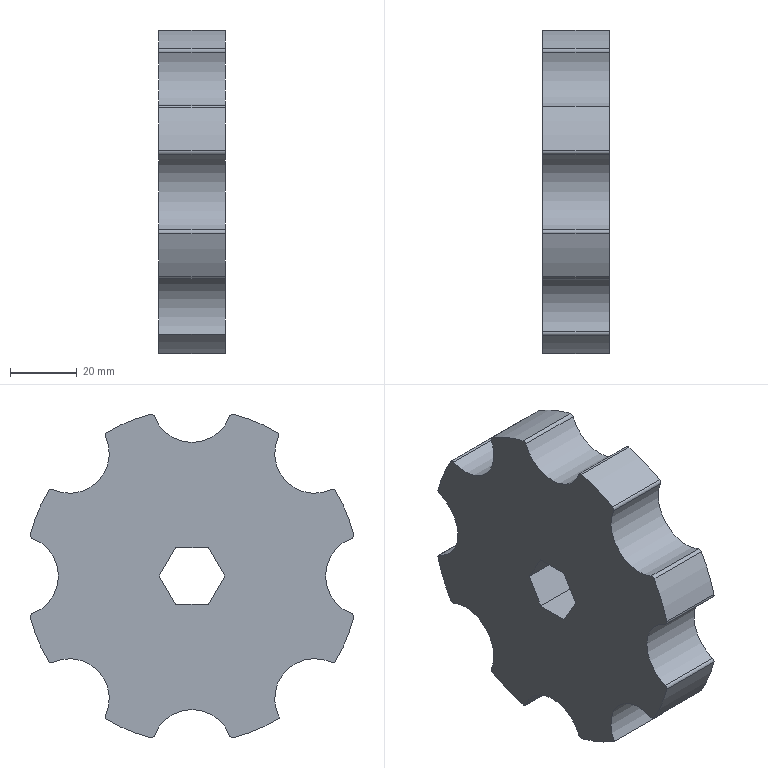Part | STEP file | Segmented slotted wheel | 1 solid | 39 faces | box 20 x 96.923 x 96.923 mm | volume 125193 mm3 | cylinder 31 | plane 8 | commonest cylinder face diameters 2 x15 24 x8 100 x8
STEP:
#1=CARTESIAN_POINT('',(20.,-48.43,-12.431));
#2=VERTEX_POINT('',#1);
#3=CARTESIAN_POINT('',(20.,-43.035,-25.455));
#4=VERTEX_POINT('',#3);
#5=CARTESIAN_POINT('',(20.,0.,0.));
#6=DIRECTION('',(1.,0.,0.));
#7=DIRECTION('',(0.,0.,-1.));
#8=AXIS2_PLACEMENT_3D('',#5,#6,#7);
#9=CIRCLE('',#8,50.);
#10=EDGE_CURVE('',#2,#4,#9,.T.);
#11=ORIENTED_EDGE('',*,*,#10,.T.);
#12=CARTESIAN_POINT('',(20.,-41.759,-25.856));
#13=VERTEX_POINT('',#12);
#14=CARTESIAN_POINT('',(20.,-42.174,-24.946));
#15=DIRECTION('',(1.,0.,0.));
#16=DIRECTION('',(0.,0.,-1.));
#17=AXIS2_PLACEMENT_3D('',#14,#15,#16);
#18=CIRCLE('',#17,1.);
#19=EDGE_CURVE('',#4,#13,#18,.T.);
#20=ORIENTED_EDGE('',*,*,#19,.T.);
#21=CARTESIAN_POINT('',(20.,-26.255,-42.552));
#22=VERTEX_POINT('',#21);
#23=CARTESIAN_POINT('',(20.,-36.77,-36.77));
#24=DIRECTION('',(-1.,0.,0.));
#25=DIRECTION('',(0.,0.,-1.));
#26=AXIS2_PLACEMENT_3D('',#23,#24,#25);
#27=CIRCLE('',#26,12.);
#28=EDGE_CURVE('',#13,#22,#27,.T.);
#29=ORIENTED_EDGE('',*,*,#28,.T.);
#30=CARTESIAN_POINT('',(20.,-12.431,-48.43));
#31=VERTEX_POINT('',#30);
#32=CARTESIAN_POINT('',(20.,0.,0.));
#33=DIRECTION('',(1.,0.,0.));
#34=DIRECTION('',(0.,0.,-1.));
#35=AXIS2_PLACEMENT_3D('',#32,#33,#34);
#36=CIRCLE('',#35,50.);
#37=EDGE_CURVE('',#22,#31,#36,.T.);
#38=ORIENTED_EDGE('',*,*,#37,.T.);
#39=CARTESIAN_POINT('',(20.,-11.245,-47.811));
#40=VERTEX_POINT('',#39);
#41=CARTESIAN_POINT('',(20.,-12.182,-47.462));
#42=DIRECTION('',(1.,0.,0.));
#43=DIRECTION('',(0.,0.,-1.));
#44=AXIS2_PLACEMENT_3D('',#41,#42,#43);
#45=CIRCLE('',#44,1.);
#46=EDGE_CURVE('',#31,#40,#45,.T.);
#47=ORIENTED_EDGE('',*,*,#46,.T.);
#48=CARTESIAN_POINT('',(20.,11.245,-47.811));
#49=VERTEX_POINT('',#48);
#50=CARTESIAN_POINT('',(20.,0.,-52.));
#51=DIRECTION('',(-1.,0.,0.));
#52=DIRECTION('',(0.,0.,-1.));
#53=AXIS2_PLACEMENT_3D('',#50,#51,#52);
#54=CIRCLE('',#53,12.);
#55=EDGE_CURVE('',#40,#49,#54,.T.);
#56=ORIENTED_EDGE('',*,*,#55,.T.);
#57=CARTESIAN_POINT('',(20.,12.431,-48.43));
#58=VERTEX_POINT('',#57);
#59=CARTESIAN_POINT('',(20.,12.182,-47.462));
#60=DIRECTION('',(1.,0.,0.));
#61=DIRECTION('',(0.,0.,-1.));
#62=AXIS2_PLACEMENT_3D('',#59,#60,#61);
#63=CIRCLE('',#62,1.);
#64=EDGE_CURVE('',#49,#58,#63,.T.);
#65=ORIENTED_EDGE('',*,*,#64,.T.);
#66=CARTESIAN_POINT('',(20.,25.455,-43.035));
#67=VERTEX_POINT('',#66);
#68=CARTESIAN_POINT('',(20.,0.,0.));
#69=DIRECTION('',(1.,0.,0.));
#70=DIRECTION('',(0.,0.,-1.));
#71=AXIS2_PLACEMENT_3D('',#68,#69,#70);
#72=CIRCLE('',#71,50.);
#73=EDGE_CURVE('',#58,#67,#72,.T.);
#74=ORIENTED_EDGE('',*,*,#73,.T.);
#75=CARTESIAN_POINT('',(20.,25.856,-41.759));
#76=VERTEX_POINT('',#75);
#77=CARTESIAN_POINT('',(20.,24.946,-42.174));
#78=DIRECTION('',(1.,0.,0.));
#79=DIRECTION('',(0.,0.,-1.));
#80=AXIS2_PLACEMENT_3D('',#77,#78,#79);
#81=CIRCLE('',#80,1.);
#82=EDGE_CURVE('',#67,#76,#81,.T.);
#83=ORIENTED_EDGE('',*,*,#82,.T.);
#84=CARTESIAN_POINT('',(20.,41.759,-25.856));
#85=VERTEX_POINT('',#84);
#86=CARTESIAN_POINT('',(20.,36.77,-36.77));
#87=DIRECTION('',(-1.,0.,0.));
#88=DIRECTION('',(0.,0.,-1.));
#89=AXIS2_PLACEMENT_3D('',#86,#87,#88);
#90=CIRCLE('',#89,12.);
#91=EDGE_CURVE('',#76,#85,#90,.T.);
#92=ORIENTED_EDGE('',*,*,#91,.T.);
#93=CARTESIAN_POINT('',(20.,43.035,-25.455));
#94=VERTEX_POINT('',#93);
#95=CARTESIAN_POINT('',(20.,42.174,-24.946));
#96=DIRECTION('',(1.,0.,0.));
#97=DIRECTION('',(0.,0.,-1.));
#98=AXIS2_PLACEMENT_3D('',#95,#96,#97);
#99=CIRCLE('',#98,1.);
#100=EDGE_CURVE('',#85,#94,#99,.T.);
#101=ORIENTED_EDGE('',*,*,#100,.T.);
#102=CARTESIAN_POINT('',(20.,48.43,-12.431));
#103=VERTEX_POINT('',#102);
#104=CARTESIAN_POINT('',(20.,0.,0.));
#105=DIRECTION('',(1.,0.,0.));
#106=DIRECTION('',(0.,0.,-1.));
#107=AXIS2_PLACEMENT_3D('',#104,#105,#106);
#108=CIRCLE('',#107,50.);
#109=EDGE_CURVE('',#94,#103,#108,.T.);
#110=ORIENTED_EDGE('',*,*,#109,.T.);
#111=CARTESIAN_POINT('',(20.,47.811,-11.245));
#112=VERTEX_POINT('',#111);
#113=CARTESIAN_POINT('',(20.,47.462,-12.182));
#114=DIRECTION('',(1.,0.,0.));
#115=DIRECTION('',(0.,0.,-1.));
#116=AXIS2_PLACEMENT_3D('',#113,#114,#115);
#117=CIRCLE('',#116,1.);
#118=EDGE_CURVE('',#103,#112,#117,.T.);
#119=ORIENTED_EDGE('',*,*,#118,.T.);
#120=CARTESIAN_POINT('',(20.,47.811,11.245));
#121=VERTEX_POINT('',#120);
#122=CARTESIAN_POINT('',(20.,52.,0.));
#123=DIRECTION('',(-1.,0.,0.));
#124=DIRECTION('',(0.,0.,-1.));
#125=AXIS2_PLACEMENT_3D('',#122,#123,#124);
#126=CIRCLE('',#125,12.);
#127=EDGE_CURVE('',#112,#121,#126,.T.);
#128=ORIENTED_EDGE('',*,*,#127,.T.);
#129=CARTESIAN_POINT('',(20.,48.43,12.431));
#130=VERTEX_POINT('',#129);
#131=CARTESIAN_POINT('',(20.,47.462,12.182));
#132=DIRECTION('',(1.,0.,0.));
#133=DIRECTION('',(0.,0.,-1.));
#134=AXIS2_PLACEMENT_3D('',#131,#132,#133);
#135=CIRCLE('',#134,1.);
#136=EDGE_CURVE('',#121,#130,#135,.T.);
#137=ORIENTED_EDGE('',*,*,#136,.T.);
#138=CARTESIAN_POINT('',(20.,43.035,25.455));
#139=VERTEX_POINT('',#138);
#140=CARTESIAN_POINT('',(20.,0.,0.));
#141=DIRECTION('',(1.,0.,0.));
#142=DIRECTION('',(0.,0.,-1.));
#143=AXIS2_PLACEMENT_3D('',#140,#141,#142);
#144=CIRCLE('',#143,50.);
#145=EDGE_CURVE('',#130,#139,#144,.T.);
#146=ORIENTED_EDGE('',*,*,#145,.T.);
#147=CARTESIAN_POINT('',(20.,41.759,25.856));
#148=VERTEX_POINT('',#147);
#149=CARTESIAN_POINT('',(20.,42.174,24.946));
#150=DIRECTION('',(1.,0.,0.));
#151=DIRECTION('',(0.,0.,-1.));
#152=AXIS2_PLACEMENT_3D('',#149,#150,#151);
#153=CIRCLE('',#152,1.);
#154=EDGE_CURVE('',#139,#148,#153,.T.);
#155=ORIENTED_EDGE('',*,*,#154,.T.);
#156=CARTESIAN_POINT('',(20.,25.856,41.759));
#157=VERTEX_POINT('',#156);
#158=CARTESIAN_POINT('',(20.,36.77,36.77));
#159=DIRECTION('',(-1.,0.,0.));
#160=DIRECTION('',(0.,0.,-1.));
#161=AXIS2_PLACEMENT_3D('',#158,#159,#160);
#162=CIRCLE('',#161,12.);
#163=EDGE_CURVE('',#148,#157,#162,.T.);
#164=ORIENTED_EDGE('',*,*,#163,.T.);
#165=CARTESIAN_POINT('',(20.,25.455,43.035));
#166=VERTEX_POINT('',#165);
#167=CARTESIAN_POINT('',(20.,24.946,42.174));
#168=DIRECTION('',(1.,0.,0.));
#169=DIRECTION('',(0.,0.,-1.));
#170=AXIS2_PLACEMENT_3D('',#167,#168,#169);
#171=CIRCLE('',#170,1.);
#172=EDGE_CURVE('',#157,#166,#171,.T.);
#173=ORIENTED_EDGE('',*,*,#172,.T.);
#174=CARTESIAN_POINT('',(20.,12.431,48.43));
#175=VERTEX_POINT('',#174);
#176=CARTESIAN_POINT('',(20.,0.,0.));
#177=DIRECTION('',(1.,0.,0.));
#178=DIRECTION('',(0.,0.,-1.));
#179=AXIS2_PLACEMENT_3D('',#176,#177,#178);
#180=CIRCLE('',#179,50.);
#181=EDGE_CURVE('',#166,#175,#180,.T.);
#182=ORIENTED_EDGE('',*,*,#181,.T.);
#183=CARTESIAN_POINT('',(20.,11.245,47.811));
#184=VERTEX_POINT('',#183);
#185=CARTESIAN_POINT('',(20.,12.182,47.462));
#186=DIRECTION('',(1.,0.,0.));
#187=DIRECTION('',(0.,0.,-1.));
#188=AXIS2_PLACEMENT_3D('',#185,#186,#187);
#189=CIRCLE('',#188,1.);
#190=EDGE_CURVE('',#175,#184,#189,.T.);
#191=ORIENTED_EDGE('',*,*,#190,.T.);
#192=CARTESIAN_POINT('',(20.,-11.245,47.811));
#193=VERTEX_POINT('',#192);
#194=CARTESIAN_POINT('',(20.,0.,52.));
#195=DIRECTION('',(-1.,0.,0.));
#196=DIRECTION('',(0.,0.,-1.));
#197=AXIS2_PLACEMENT_3D('',#194,#195,#196);
#198=CIRCLE('',#197,12.);
#199=EDGE_CURVE('',#184,#193,#198,.T.);
#200=ORIENTED_EDGE('',*,*,#199,.T.);
#201=CARTESIAN_POINT('',(20.,-12.431,48.43));
#202=VERTEX_POINT('',#201);
#203=CARTESIAN_POINT('',(20.,-12.182,47.462));
#204=DIRECTION('',(1.,0.,0.));
#205=DIRECTION('',(0.,0.,-1.));
#206=AXIS2_PLACEMENT_3D('',#203,#204,#205);
#207=CIRCLE('',#206,1.);
#208=EDGE_CURVE('',#193,#202,#207,.T.);
#209=ORIENTED_EDGE('',*,*,#208,.T.);
#210=CARTESIAN_POINT('',(20.,-25.455,43.035));
#211=VERTEX_POINT('',#210);
#212=CARTESIAN_POINT('',(20.,0.,0.));
#213=DIRECTION('',(1.,0.,0.));
#214=DIRECTION('',(0.,0.,-1.));
#215=AXIS2_PLACEMENT_3D('',#212,#213,#214);
#216=CIRCLE('',#215,50.);
#217=EDGE_CURVE('',#202,#211,#216,.T.);
#218=ORIENTED_EDGE('',*,*,#217,.T.);
#219=CARTESIAN_POINT('',(20.,-25.856,41.759));
#220=VERTEX_POINT('',#219);
#221=CARTESIAN_POINT('',(20.,-24.946,42.174));
#222=DIRECTION('',(1.,0.,0.));
#223=DIRECTION('',(0.,0.,-1.));
#224=AXIS2_PLACEMENT_3D('',#221,#222,#223);
#225=CIRCLE('',#224,1.);
#226=EDGE_CURVE('',#211,#220,#225,.T.);
#227=ORIENTED_EDGE('',*,*,#226,.T.);
#228=CARTESIAN_POINT('',(20.,-41.759,25.856));
#229=VERTEX_POINT('',#228);
#230=CARTESIAN_POINT('',(20.,-36.77,36.77));
#231=DIRECTION('',(-1.,0.,0.));
#232=DIRECTION('',(0.,0.,-1.));
#233=AXIS2_PLACEMENT_3D('',#230,#231,#232);
#234=CIRCLE('',#233,12.);
#235=EDGE_CURVE('',#220,#229,#234,.T.);
#236=ORIENTED_EDGE('',*,*,#235,.T.);
#237=CARTESIAN_POINT('',(20.,-43.035,25.455));
#238=VERTEX_POINT('',#237);
#239=CARTESIAN_POINT('',(20.,-42.174,24.946));
#240=DIRECTION('',(1.,0.,0.));
#241=DIRECTION('',(0.,0.,-1.));
#242=AXIS2_PLACEMENT_3D('',#239,#240,#241);
#243=CIRCLE('',#242,1.);
#244=EDGE_CURVE('',#229,#238,#243,.T.);
#245=ORIENTED_EDGE('',*,*,#244,.T.);
#246=CARTESIAN_POINT('',(20.,-48.43,12.431));
#247=VERTEX_POINT('',#246);
#248=CARTESIAN_POINT('',(20.,0.,0.));
#249=DIRECTION('',(1.,0.,0.));
#250=DIRECTION('',(0.,0.,-1.));
#251=AXIS2_PLACEMENT_3D('',#248,#249,#250);
#252=CIRCLE('',#251,50.);
#253=EDGE_CURVE('',#238,#247,#252,.T.);
#254=ORIENTED_EDGE('',*,*,#253,.T.);
#255=CARTESIAN_POINT('',(20.,-47.811,11.245));
#256=VERTEX_POINT('',#255);
#257=CARTESIAN_POINT('',(20.,-47.462,12.182));
#258=DIRECTION('',(1.,0.,0.));
#259=DIRECTION('',(0.,0.,-1.));
#260=AXIS2_PLACEMENT_3D('',#257,#258,#259);
#261=CIRCLE('',#260,1.);
#262=EDGE_CURVE('',#247,#256,#261,.T.);
#263=ORIENTED_EDGE('',*,*,#262,.T.);
#264=CARTESIAN_POINT('',(20.,-47.811,-11.245));
#265=VERTEX_POINT('',#264);
#266=CARTESIAN_POINT('',(20.,-52.,0.));
#267=DIRECTION('',(-1.,0.,0.));
#268=DIRECTION('',(0.,0.,-1.));
#269=AXIS2_PLACEMENT_3D('',#266,#267,#268);
#270=CIRCLE('',#269,12.);
#271=EDGE_CURVE('',#256,#265,#270,.T.);
#272=ORIENTED_EDGE('',*,*,#271,.T.);
#273=CARTESIAN_POINT('',(20.,-47.462,-12.182));
#274=DIRECTION('',(1.,0.,0.));
#275=DIRECTION('',(0.,0.,-1.));
#276=AXIS2_PLACEMENT_3D('',#273,#274,#275);
#277=CIRCLE('',#276,1.);
#278=EDGE_CURVE('',#265,#2,#277,.T.);
#279=ORIENTED_EDGE('',*,*,#278,.T.);
#280=EDGE_LOOP('',(#11,#20,#29,#38,#47,#56,#65,#74,#83,#92,#101,#110,#119,#128,#137,#146,#155,#164,#173,#182,#191,#200,#209,#218,#227,#236,#245,#254,#263,#272,#279));
#281=FACE_OUTER_BOUND('',#280,.T.);
#282=CARTESIAN_POINT('',(20.,9.815,0.));
#283=VERTEX_POINT('',#282);
#284=CARTESIAN_POINT('',(20.,4.907,8.5));
#285=VERTEX_POINT('',#284);
#286=CARTESIAN_POINT('',(20.,9.815,0.));
#287=DIRECTION('',(0.,-0.5,0.866));
#288=VECTOR('',#287,1000.);
#289=LINE('',#286,#288);
#290=EDGE_CURVE('',#283,#285,#289,.T.);
#291=ORIENTED_EDGE('',*,*,#290,.F.);
#292=CARTESIAN_POINT('',(20.,4.907,-8.5));
#293=VERTEX_POINT('',#292);
#294=CARTESIAN_POINT('',(20.,4.907,-8.5));
#295=DIRECTION('',(0.,0.5,0.866));
#296=VECTOR('',#295,1000.);
#297=LINE('',#294,#296);
#298=EDGE_CURVE('',#293,#283,#297,.T.);
#299=ORIENTED_EDGE('',*,*,#298,.F.);
#300=CARTESIAN_POINT('',(20.,-4.907,-8.5));
#301=VERTEX_POINT('',#300);
#302=CARTESIAN_POINT('',(20.,-4.907,-8.5));
#303=DIRECTION('',(0.,1.,0.));
#304=VECTOR('',#303,1000.);
#305=LINE('',#302,#304);
#306=EDGE_CURVE('',#301,#293,#305,.T.);
#307=ORIENTED_EDGE('',*,*,#306,.F.);
#308=CARTESIAN_POINT('',(20.,-9.815,0.));
#309=VERTEX_POINT('',#308);
#310=CARTESIAN_POINT('',(20.,-9.815,0.));
#311=DIRECTION('',(0.,0.5,-0.866));
#312=VECTOR('',#311,1000.);
#313=LINE('',#310,#312);
#314=EDGE_CURVE('',#309,#301,#313,.T.);
#315=ORIENTED_EDGE('',*,*,#314,.F.);
#316=CARTESIAN_POINT('',(20.,-4.907,8.5));
#317=VERTEX_POINT('',#316);
#318=CARTESIAN_POINT('',(20.,-4.907,8.5));
#319=DIRECTION('',(0.,-0.5,-0.866));
#320=VECTOR('',#319,1000.);
#321=LINE('',#318,#320);
#322=EDGE_CURVE('',#317,#309,#321,.T.);
#323=ORIENTED_EDGE('',*,*,#322,.F.);
#324=CARTESIAN_POINT('',(20.,4.907,8.5));
#325=DIRECTION('',(0.,-1.,0.));
#326=VECTOR('',#325,1000.);
#327=LINE('',#324,#326);
#328=EDGE_CURVE('',#285,#317,#327,.T.);
#329=ORIENTED_EDGE('',*,*,#328,.F.);
#330=EDGE_LOOP('',(#291,#299,#307,#315,#323,#329));
#331=FACE_BOUND('',#330,.T.);
#332=CARTESIAN_POINT('',(20.,26.,0.));
#333=DIRECTION('',(1.,0.,0.));
#334=DIRECTION('',(0.,0.,-1.));
#335=AXIS2_PLACEMENT_3D('',#332,#333,#334);
#336=PLANE('',#335);
#337=ADVANCED_FACE('',(#281,#331),#336,.T.);
#338=CARTESIAN_POINT('',(0.,-41.759,-25.856));
#339=VERTEX_POINT('',#338);
#340=CARTESIAN_POINT('',(0.,-26.255,-42.552));
#341=VERTEX_POINT('',#340);
#342=CARTESIAN_POINT('',(0.,-36.77,-36.77));
#343=DIRECTION('',(-1.,0.,0.));
#344=DIRECTION('',(0.,0.,-1.));
#345=AXIS2_PLACEMENT_3D('',#342,#343,#344);
#346=CIRCLE('',#345,12.);
#347=EDGE_CURVE('',#339,#341,#346,.T.);
#348=ORIENTED_EDGE('',*,*,#347,.F.);
#349=CARTESIAN_POINT('',(0.,-43.035,-25.455));
#350=VERTEX_POINT('',#349);
#351=CARTESIAN_POINT('',(0.,-42.174,-24.946));
#352=DIRECTION('',(-1.,0.,0.));
#353=DIRECTION('',(0.,0.,-1.));
#354=AXIS2_PLACEMENT_3D('',#351,#352,#353);
#355=CIRCLE('',#354,1.);
#356=EDGE_CURVE('',#339,#350,#355,.T.);
#357=ORIENTED_EDGE('',*,*,#356,.T.);
#358=CARTESIAN_POINT('',(0.,-48.43,-12.431));
#359=VERTEX_POINT('',#358);
#360=CARTESIAN_POINT('',(0.,0.,0.));
#361=DIRECTION('',(1.,0.,0.));
#362=DIRECTION('',(0.,0.,-1.));
#363=AXIS2_PLACEMENT_3D('',#360,#361,#362);
#364=CIRCLE('',#363,50.);
#365=EDGE_CURVE('',#359,#350,#364,.T.);
#366=ORIENTED_EDGE('',*,*,#365,.F.);
#367=CARTESIAN_POINT('',(0.,-47.811,-11.245));
#368=VERTEX_POINT('',#367);
#369=CARTESIAN_POINT('',(0.,-47.462,-12.182));
#370=DIRECTION('',(-1.,0.,0.));
#371=DIRECTION('',(0.,0.,-1.));
#372=AXIS2_PLACEMENT_3D('',#369,#370,#371);
#373=CIRCLE('',#372,1.);
#374=EDGE_CURVE('',#359,#368,#373,.T.);
#375=ORIENTED_EDGE('',*,*,#374,.T.);
#376=CARTESIAN_POINT('',(0.,-47.811,11.245));
#377=VERTEX_POINT('',#376);
#378=CARTESIAN_POINT('',(0.,-52.,0.));
#379=DIRECTION('',(-1.,0.,0.));
#380=DIRECTION('',(0.,0.,-1.));
#381=AXIS2_PLACEMENT_3D('',#378,#379,#380);
#382=CIRCLE('',#381,12.);
#383=EDGE_CURVE('',#377,#368,#382,.T.);
#384=ORIENTED_EDGE('',*,*,#383,.F.);
#385=CARTESIAN_POINT('',(0.,-48.43,12.431));
#386=VERTEX_POINT('',#385);
#387=CARTESIAN_POINT('',(0.,-47.462,12.182));
#388=DIRECTION('',(-1.,0.,0.));
#389=DIRECTION('',(0.,0.,-1.));
#390=AXIS2_PLACEMENT_3D('',#387,#388,#389);
#391=CIRCLE('',#390,1.);
#392=EDGE_CURVE('',#377,#386,#391,.T.);
#393=ORIENTED_EDGE('',*,*,#392,.T.);
#394=CARTESIAN_POINT('',(0.,-43.035,25.455));
#395=VERTEX_POINT('',#394);
#396=CARTESIAN_POINT('',(0.,0.,0.));
#397=DIRECTION('',(1.,0.,0.));
#398=DIRECTION('',(0.,0.,-1.));
#399=AXIS2_PLACEMENT_3D('',#396,#397,#398);
#400=CIRCLE('',#399,50.);
#401=EDGE_CURVE('',#395,#386,#400,.T.);
#402=ORIENTED_EDGE('',*,*,#401,.F.);
#403=CARTESIAN_POINT('',(0.,-41.759,25.856));
#404=VERTEX_POINT('',#403);
#405=CARTESIAN_POINT('',(0.,-42.174,24.946));
#406=DIRECTION('',(-1.,0.,0.));
#407=DIRECTION('',(0.,0.,-1.));
#408=AXIS2_PLACEMENT_3D('',#405,#406,#407);
#409=CIRCLE('',#408,1.);
#410=EDGE_CURVE('',#395,#404,#409,.T.);
#411=ORIENTED_EDGE('',*,*,#410,.T.);
#412=CARTESIAN_POINT('',(0.,-25.856,41.759));
#413=VERTEX_POINT('',#412);
#414=CARTESIAN_POINT('',(0.,-36.77,36.77));
#415=DIRECTION('',(-1.,0.,0.));
#416=DIRECTION('',(0.,0.,-1.));
#417=AXIS2_PLACEMENT_3D('',#414,#415,#416);
#418=CIRCLE('',#417,12.);
#419=EDGE_CURVE('',#413,#404,#418,.T.);
#420=ORIENTED_EDGE('',*,*,#419,.F.);
#421=CARTESIAN_POINT('',(0.,-25.455,43.035));
#422=VERTEX_POINT('',#421);
#423=CARTESIAN_POINT('',(0.,-24.946,42.174));
#424=DIRECTION('',(-1.,0.,0.));
#425=DIRECTION('',(0.,0.,-1.));
#426=AXIS2_PLACEMENT_3D('',#423,#424,#425);
#427=CIRCLE('',#426,1.);
#428=EDGE_CURVE('',#413,#422,#427,.T.);
#429=ORIENTED_EDGE('',*,*,#428,.T.);
#430=CARTESIAN_POINT('',(0.,-12.431,48.43));
#431=VERTEX_POINT('',#430);
#432=CARTESIAN_POINT('',(0.,0.,0.));
#433=DIRECTION('',(1.,0.,0.));
#434=DIRECTION('',(0.,0.,-1.));
#435=AXIS2_PLACEMENT_3D('',#432,#433,#434);
#436=CIRCLE('',#435,50.);
#437=EDGE_CURVE('',#431,#422,#436,.T.);
#438=ORIENTED_EDGE('',*,*,#437,.F.);
#439=CARTESIAN_POINT('',(0.,-11.245,47.811));
#440=VERTEX_POINT('',#439);
#441=CARTESIAN_POINT('',(0.,-12.182,47.462));
#442=DIRECTION('',(-1.,0.,0.));
#443=DIRECTION('',(0.,0.,-1.));
#444=AXIS2_PLACEMENT_3D('',#441,#442,#443);
#445=CIRCLE('',#444,1.);
#446=EDGE_CURVE('',#431,#440,#445,.T.);
#447=ORIENTED_EDGE('',*,*,#446,.T.);
#448=CARTESIAN_POINT('',(0.,11.245,47.811));
#449=VERTEX_POINT('',#448);
#450=CARTESIAN_POINT('',(0.,0.,52.));
#451=DIRECTION('',(-1.,0.,0.));
#452=DIRECTION('',(0.,0.,-1.));
#453=AXIS2_PLACEMENT_3D('',#450,#451,#452);
#454=CIRCLE('',#453,12.);
#455=EDGE_CURVE('',#449,#440,#454,.T.);
#456=ORIENTED_EDGE('',*,*,#455,.F.);
#457=CARTESIAN_POINT('',(0.,12.431,48.43));
#458=VERTEX_POINT('',#457);
#459=CARTESIAN_POINT('',(0.,12.182,47.462));
#460=DIRECTION('',(-1.,0.,0.));
#461=DIRECTION('',(0.,0.,-1.));
#462=AXIS2_PLACEMENT_3D('',#459,#460,#461);
#463=CIRCLE('',#462,1.);
#464=EDGE_CURVE('',#449,#458,#463,.T.);
#465=ORIENTED_EDGE('',*,*,#464,.T.);
#466=CARTESIAN_POINT('',(0.,25.455,43.035));
#467=VERTEX_POINT('',#466);
#468=CARTESIAN_POINT('',(0.,0.,0.));
#469=DIRECTION('',(1.,0.,0.));
#470=DIRECTION('',(0.,0.,-1.));
#471=AXIS2_PLACEMENT_3D('',#468,#469,#470);
#472=CIRCLE('',#471,50.);
#473=EDGE_CURVE('',#467,#458,#472,.T.);
#474=ORIENTED_EDGE('',*,*,#473,.F.);
#475=CARTESIAN_POINT('',(0.,25.856,41.759));
#476=VERTEX_POINT('',#475);
#477=CARTESIAN_POINT('',(0.,24.946,42.174));
#478=DIRECTION('',(-1.,0.,0.));
#479=DIRECTION('',(0.,0.,-1.));
#480=AXIS2_PLACEMENT_3D('',#477,#478,#479);
#481=CIRCLE('',#480,1.);
#482=EDGE_CURVE('',#467,#476,#481,.T.);
#483=ORIENTED_EDGE('',*,*,#482,.T.);
#484=CARTESIAN_POINT('',(0.,41.759,25.856));
#485=VERTEX_POINT('',#484);
#486=CARTESIAN_POINT('',(0.,36.77,36.77));
#487=DIRECTION('',(-1.,0.,0.));
#488=DIRECTION('',(0.,0.,-1.));
#489=AXIS2_PLACEMENT_3D('',#486,#487,#488);
#490=CIRCLE('',#489,12.);
#491=EDGE_CURVE('',#485,#476,#490,.T.);
#492=ORIENTED_EDGE('',*,*,#491,.F.);
#493=CARTESIAN_POINT('',(0.,43.035,25.455));
#494=VERTEX_POINT('',#493);
#495=CARTESIAN_POINT('',(0.,42.174,24.946));
#496=DIRECTION('',(-1.,0.,0.));
#497=DIRECTION('',(0.,0.,-1.));
#498=AXIS2_PLACEMENT_3D('',#495,#496,#497);
#499=CIRCLE('',#498,1.);
#500=EDGE_CURVE('',#485,#494,#499,.T.);
#501=ORIENTED_EDGE('',*,*,#500,.T.);
#502=CARTESIAN_POINT('',(0.,48.43,12.431));
#503=VERTEX_POINT('',#502);
#504=CARTESIAN_POINT('',(0.,0.,0.));
#505=DIRECTION('',(1.,0.,0.));
#506=DIRECTION('',(0.,0.,-1.));
#507=AXIS2_PLACEMENT_3D('',#504,#505,#506);
#508=CIRCLE('',#507,50.);
#509=EDGE_CURVE('',#503,#494,#508,.T.);
#510=ORIENTED_EDGE('',*,*,#509,.F.);
#511=CARTESIAN_POINT('',(0.,47.811,11.245));
#512=VERTEX_POINT('',#511);
#513=CARTESIAN_POINT('',(0.,47.462,12.182));
#514=DIRECTION('',(-1.,0.,0.));
#515=DIRECTION('',(0.,0.,-1.));
#516=AXIS2_PLACEMENT_3D('',#513,#514,#515);
#517=CIRCLE('',#516,1.);
#518=EDGE_CURVE('',#503,#512,#517,.T.);
#519=ORIENTED_EDGE('',*,*,#518,.T.);
#520=CARTESIAN_POINT('',(0.,47.811,-11.245));
#521=VERTEX_POINT('',#520);
#522=CARTESIAN_POINT('',(0.,52.,0.));
#523=DIRECTION('',(-1.,0.,0.));
#524=DIRECTION('',(0.,0.,-1.));
#525=AXIS2_PLACEMENT_3D('',#522,#523,#524);
#526=CIRCLE('',#525,12.);
#527=EDGE_CURVE('',#521,#512,#526,.T.);
#528=ORIENTED_EDGE('',*,*,#527,.F.);
#529=CARTESIAN_POINT('',(0.,48.43,-12.431));
#530=VERTEX_POINT('',#529);
#531=CARTESIAN_POINT('',(0.,47.462,-12.182));
#532=DIRECTION('',(-1.,0.,0.));
#533=DIRECTION('',(0.,0.,-1.));
#534=AXIS2_PLACEMENT_3D('',#531,#532,#533);
#535=CIRCLE('',#534,1.);
#536=EDGE_CURVE('',#521,#530,#535,.T.);
#537=ORIENTED_EDGE('',*,*,#536,.T.);
#538=CARTESIAN_POINT('',(0.,43.035,-25.455));
#539=VERTEX_POINT('',#538);
#540=CARTESIAN_POINT('',(0.,0.,0.));
#541=DIRECTION('',(1.,0.,0.));
#542=DIRECTION('',(0.,0.,-1.));
#543=AXIS2_PLACEMENT_3D('',#540,#541,#542);
#544=CIRCLE('',#543,50.);
#545=EDGE_CURVE('',#539,#530,#544,.T.);
#546=ORIENTED_EDGE('',*,*,#545,.F.);
#547=CARTESIAN_POINT('',(0.,41.759,-25.856));
#548=VERTEX_POINT('',#547);
#549=CARTESIAN_POINT('',(0.,42.174,-24.946));
#550=DIRECTION('',(-1.,0.,0.));
#551=DIRECTION('',(0.,0.,-1.));
#552=AXIS2_PLACEMENT_3D('',#549,#550,#551);
#553=CIRCLE('',#552,1.);
#554=EDGE_CURVE('',#539,#548,#553,.T.);
#555=ORIENTED_EDGE('',*,*,#554,.T.);
#556=CARTESIAN_POINT('',(0.,25.856,-41.759));
#557=VERTEX_POINT('',#556);
#558=CARTESIAN_POINT('',(0.,36.77,-36.77));
#559=DIRECTION('',(-1.,0.,0.));
#560=DIRECTION('',(0.,0.,-1.));
#561=AXIS2_PLACEMENT_3D('',#558,#559,#560);
#562=CIRCLE('',#561,12.);
#563=EDGE_CURVE('',#557,#548,#562,.T.);
#564=ORIENTED_EDGE('',*,*,#563,.F.);
#565=CARTESIAN_POINT('',(0.,25.455,-43.035));
#566=VERTEX_POINT('',#565);
#567=CARTESIAN_POINT('',(0.,24.946,-42.174));
#568=DIRECTION('',(-1.,0.,0.));
#569=DIRECTION('',(0.,0.,-1.));
#570=AXIS2_PLACEMENT_3D('',#567,#568,#569);
#571=CIRCLE('',#570,1.);
#572=EDGE_CURVE('',#557,#566,#571,.T.);
#573=ORIENTED_EDGE('',*,*,#572,.T.);
#574=CARTESIAN_POINT('',(0.,12.431,-48.43));
#575=VERTEX_POINT('',#574);
#576=CARTESIAN_POINT('',(0.,0.,0.));
#577=DIRECTION('',(1.,0.,0.));
#578=DIRECTION('',(0.,0.,-1.));
#579=AXIS2_PLACEMENT_3D('',#576,#577,#578);
#580=CIRCLE('',#579,50.);
#581=EDGE_CURVE('',#575,#566,#580,.T.);
#582=ORIENTED_EDGE('',*,*,#581,.F.);
#583=CARTESIAN_POINT('',(0.,11.245,-47.811));
#584=VERTEX_POINT('',#583);
#585=CARTESIAN_POINT('',(0.,12.182,-47.462));
#586=DIRECTION('',(-1.,0.,0.));
#587=DIRECTION('',(0.,0.,-1.));
#588=AXIS2_PLACEMENT_3D('',#585,#586,#587);
#589=CIRCLE('',#588,1.);
#590=EDGE_CURVE('',#575,#584,#589,.T.);
#591=ORIENTED_EDGE('',*,*,#590,.T.);
#592=CARTESIAN_POINT('',(0.,-11.245,-47.811));
#593=VERTEX_POINT('',#592);
#594=CARTESIAN_POINT('',(0.,0.,-52.));
#595=DIRECTION('',(-1.,0.,0.));
#596=DIRECTION('',(0.,0.,-1.));
#597=AXIS2_PLACEMENT_3D('',#594,#595,#596);
#598=CIRCLE('',#597,12.);
#599=EDGE_CURVE('',#593,#584,#598,.T.);
#600=ORIENTED_EDGE('',*,*,#599,.F.);
#601=CARTESIAN_POINT('',(0.,-12.431,-48.43));
#602=VERTEX_POINT('',#601);
#603=CARTESIAN_POINT('',(0.,-12.182,-47.462));
#604=DIRECTION('',(-1.,0.,0.));
#605=DIRECTION('',(0.,0.,-1.));
#606=AXIS2_PLACEMENT_3D('',#603,#604,#605);
#607=CIRCLE('',#606,1.);
#608=EDGE_CURVE('',#593,#602,#607,.T.);
#609=ORIENTED_EDGE('',*,*,#608,.T.);
#610=CARTESIAN_POINT('',(0.,0.,0.));
#611=DIRECTION('',(1.,0.,0.));
#612=DIRECTION('',(0.,0.,-1.));
#613=AXIS2_PLACEMENT_3D('',#610,#611,#612);
#614=CIRCLE('',#613,50.);
#615=EDGE_CURVE('',#341,#602,#614,.T.);
#616=ORIENTED_EDGE('',*,*,#615,.F.);
#617=EDGE_LOOP('',(#348,#357,#366,#375,#384,#393,#402,#411,#420,#429,#438,#447,#456,#465,#474,#483,#492,#501,#510,#519,#528,#537,#546,#555,#564,#573,#582,#591,#600,#609,#616));
#618=FACE_OUTER_BOUND('',#617,.T.);
#619=CARTESIAN_POINT('',(0.,4.907,-8.5));
#620=VERTEX_POINT('',#619);
#621=CARTESIAN_POINT('',(0.,9.815,0.));
#622=VERTEX_POINT('',#621);
#623=CARTESIAN_POINT('',(0.,4.907,-8.5));
#624=DIRECTION('',(0.,0.5,0.866));
#625=VECTOR('',#624,1000.);
#626=LINE('',#623,#625);
#627=EDGE_CURVE('',#620,#622,#626,.T.);
#628=ORIENTED_EDGE('',*,*,#627,.T.);
#629=CARTESIAN_POINT('',(0.,4.907,8.5));
#630=VERTEX_POINT('',#629);
#631=CARTESIAN_POINT('',(0.,9.815,0.));
#632=DIRECTION('',(0.,-0.5,0.866));
#633=VECTOR('',#632,1000.);
#634=LINE('',#631,#633);
#635=EDGE_CURVE('',#622,#630,#634,.T.);
#636=ORIENTED_EDGE('',*,*,#635,.T.);
#637=CARTESIAN_POINT('',(0.,-4.907,8.5));
#638=VERTEX_POINT('',#637);
#639=CARTESIAN_POINT('',(0.,4.907,8.5));
#640=DIRECTION('',(0.,-1.,0.));
#641=VECTOR('',#640,1000.);
#642=LINE('',#639,#641);
#643=EDGE_CURVE('',#630,#638,#642,.T.);
#644=ORIENTED_EDGE('',*,*,#643,.T.);
#645=CARTESIAN_POINT('',(0.,-9.815,0.));
#646=VERTEX_POINT('',#645);
#647=CARTESIAN_POINT('',(0.,-4.907,8.5));
#648=DIRECTION('',(0.,-0.5,-0.866));
#649=VECTOR('',#648,1000.);
#650=LINE('',#647,#649);
#651=EDGE_CURVE('',#638,#646,#650,.T.);
#652=ORIENTED_EDGE('',*,*,#651,.T.);
#653=CARTESIAN_POINT('',(0.,-4.907,-8.5));
#654=VERTEX_POINT('',#653);
#655=CARTESIAN_POINT('',(0.,-9.815,0.));
#656=DIRECTION('',(0.,0.5,-0.866));
#657=VECTOR('',#656,1000.);
#658=LINE('',#655,#657);
#659=EDGE_CURVE('',#646,#654,#658,.T.);
#660=ORIENTED_EDGE('',*,*,#659,.T.);
#661=CARTESIAN_POINT('',(0.,-4.907,-8.5));
#662=DIRECTION('',(0.,1.,0.));
#663=VECTOR('',#662,1000.);
#664=LINE('',#661,#663);
#665=EDGE_CURVE('',#654,#620,#664,.T.);
#666=ORIENTED_EDGE('',*,*,#665,.T.);
#667=EDGE_LOOP('',(#628,#636,#644,#652,#660,#666));
#668=FACE_BOUND('',#667,.T.);
#669=CARTESIAN_POINT('',(0.,26.,0.));
#670=DIRECTION('',(1.,0.,0.));
#671=DIRECTION('',(0.,0.,-1.));
#672=AXIS2_PLACEMENT_3D('',#669,#670,#671);
#673=PLANE('',#672);
#674=ADVANCED_FACE('',(#618,#668),#673,.F.);
#675=ORIENTED_EDGE('',*,*,#109,.F.);
#676=CARTESIAN_POINT('',(20.,43.035,-25.455));
#677=DIRECTION('',(-1.,0.,0.));
#678=VECTOR('',#677,1000.);
#679=LINE('',#676,#678);
#680=EDGE_CURVE('',#94,#539,#679,.T.);
#681=ORIENTED_EDGE('',*,*,#680,.T.);
#682=ORIENTED_EDGE('',*,*,#545,.T.);
#683=CARTESIAN_POINT('',(20.,48.43,-12.431));
#684=DIRECTION('',(1.,0.,0.));
#685=VECTOR('',#684,1000.);
#686=LINE('',#683,#685);
#687=EDGE_CURVE('',#530,#103,#686,.T.);
#688=ORIENTED_EDGE('',*,*,#687,.T.);
#689=EDGE_LOOP('',(#675,#681,#682,#688));
#690=FACE_OUTER_BOUND('',#689,.T.);
#691=CARTESIAN_POINT('',(20.,0.,0.));
#692=DIRECTION('',(-1.,0.,0.));
#693=DIRECTION('',(0.,0.,1.));
#694=AXIS2_PLACEMENT_3D('',#691,#692,#693);
#695=CYLINDRICAL_SURFACE('',#694,50.);
#696=ADVANCED_FACE('',(#690),#695,.T.);
#697=ORIENTED_EDGE('',*,*,#127,.F.);
#698=CARTESIAN_POINT('',(20.,47.811,-11.245));
#699=DIRECTION('',(-1.,0.,0.));
#700=VECTOR('',#699,1000.);
#701=LINE('',#698,#700);
#702=EDGE_CURVE('',#112,#521,#701,.T.);
#703=ORIENTED_EDGE('',*,*,#702,.T.);
#704=ORIENTED_EDGE('',*,*,#527,.T.);
#705=CARTESIAN_POINT('',(20.,47.811,11.245));
#706=DIRECTION('',(1.,0.,0.));
#707=VECTOR('',#706,1000.);
#708=LINE('',#705,#707);
#709=EDGE_CURVE('',#512,#121,#708,.T.);
#710=ORIENTED_EDGE('',*,*,#709,.T.);
#711=EDGE_LOOP('',(#697,#703,#704,#710));
#712=FACE_OUTER_BOUND('',#711,.T.);
#713=CARTESIAN_POINT('',(20.,52.,0.));
#714=DIRECTION('',(-1.,0.,0.));
#715=DIRECTION('',(0.,0.,1.));
#716=AXIS2_PLACEMENT_3D('',#713,#714,#715);
#717=CYLINDRICAL_SURFACE('',#716,12.);
#718=ADVANCED_FACE('',(#712),#717,.F.);
#719=ORIENTED_EDGE('',*,*,#145,.F.);
#720=CARTESIAN_POINT('',(20.,48.43,12.431));
#721=DIRECTION('',(-1.,0.,0.));
#722=VECTOR('',#721,1000.);
#723=LINE('',#720,#722);
#724=EDGE_CURVE('',#130,#503,#723,.T.);
#725=ORIENTED_EDGE('',*,*,#724,.T.);
#726=ORIENTED_EDGE('',*,*,#509,.T.);
#727=CARTESIAN_POINT('',(20.,43.035,25.455));
#728=DIRECTION('',(1.,0.,0.));
#729=VECTOR('',#728,1000.);
#730=LINE('',#727,#729);
#731=EDGE_CURVE('',#494,#139,#730,.T.);
#732=ORIENTED_EDGE('',*,*,#731,.T.);
#733=EDGE_LOOP('',(#719,#725,#726,#732));
#734=FACE_OUTER_BOUND('',#733,.T.);
#735=CARTESIAN_POINT('',(20.,0.,0.));
#736=DIRECTION('',(-1.,0.,0.));
#737=DIRECTION('',(0.,0.,1.));
#738=AXIS2_PLACEMENT_3D('',#735,#736,#737);
#739=CYLINDRICAL_SURFACE('',#738,50.);
#740=ADVANCED_FACE('',(#734),#739,.T.);
#741=ORIENTED_EDGE('',*,*,#163,.F.);
#742=CARTESIAN_POINT('',(20.,41.759,25.856));
#743=DIRECTION('',(-1.,0.,0.));
#744=VECTOR('',#743,1000.);
#745=LINE('',#742,#744);
#746=EDGE_CURVE('',#148,#485,#745,.T.);
#747=ORIENTED_EDGE('',*,*,#746,.T.);
#748=ORIENTED_EDGE('',*,*,#491,.T.);
#749=CARTESIAN_POINT('',(20.,25.856,41.759));
#750=DIRECTION('',(1.,0.,0.));
#751=VECTOR('',#750,1000.);
#752=LINE('',#749,#751);
#753=EDGE_CURVE('',#476,#157,#752,.T.);
#754=ORIENTED_EDGE('',*,*,#753,.T.);
#755=EDGE_LOOP('',(#741,#747,#748,#754));
#756=FACE_OUTER_BOUND('',#755,.T.);
#757=CARTESIAN_POINT('',(20.,36.77,36.77));
#758=DIRECTION('',(-1.,0.,0.));
#759=DIRECTION('',(0.,0.,1.));
#760=AXIS2_PLACEMENT_3D('',#757,#758,#759);
#761=CYLINDRICAL_SURFACE('',#760,12.);
#762=ADVANCED_FACE('',(#756),#761,.F.);
#763=ORIENTED_EDGE('',*,*,#181,.F.);
#764=CARTESIAN_POINT('',(20.,25.455,43.035));
#765=DIRECTION('',(-1.,0.,0.));
#766=VECTOR('',#765,1000.);
#767=LINE('',#764,#766);
#768=EDGE_CURVE('',#166,#467,#767,.T.);
#769=ORIENTED_EDGE('',*,*,#768,.T.);
#770=ORIENTED_EDGE('',*,*,#473,.T.);
#771=CARTESIAN_POINT('',(20.,12.431,48.43));
#772=DIRECTION('',(1.,0.,0.));
#773=VECTOR('',#772,1000.);
#774=LINE('',#771,#773);
#775=EDGE_CURVE('',#458,#175,#774,.T.);
#776=ORIENTED_EDGE('',*,*,#775,.T.);
#777=EDGE_LOOP('',(#763,#769,#770,#776));
#778=FACE_OUTER_BOUND('',#777,.T.);
#779=CARTESIAN_POINT('',(20.,0.,0.));
#780=DIRECTION('',(-1.,0.,0.));
#781=DIRECTION('',(0.,0.,1.));
#782=AXIS2_PLACEMENT_3D('',#779,#780,#781);
#783=CYLINDRICAL_SURFACE('',#782,50.);
#784=ADVANCED_FACE('',(#778),#783,.T.);
#785=ORIENTED_EDGE('',*,*,#199,.F.);
#786=CARTESIAN_POINT('',(20.,11.245,47.811));
#787=DIRECTION('',(-1.,0.,0.));
#788=VECTOR('',#787,1000.);
#789=LINE('',#786,#788);
#790=EDGE_CURVE('',#184,#449,#789,.T.);
#791=ORIENTED_EDGE('',*,*,#790,.T.);
#792=ORIENTED_EDGE('',*,*,#455,.T.);
#793=CARTESIAN_POINT('',(20.,-11.245,47.811));
#794=DIRECTION('',(1.,0.,0.));
#795=VECTOR('',#794,1000.);
#796=LINE('',#793,#795);
#797=EDGE_CURVE('',#440,#193,#796,.T.);
#798=ORIENTED_EDGE('',*,*,#797,.T.);
#799=EDGE_LOOP('',(#785,#791,#792,#798));
#800=FACE_OUTER_BOUND('',#799,.T.);
#801=CARTESIAN_POINT('',(20.,0.,52.));
#802=DIRECTION('',(-1.,0.,0.));
#803=DIRECTION('',(0.,0.,1.));
#804=AXIS2_PLACEMENT_3D('',#801,#802,#803);
#805=CYLINDRICAL_SURFACE('',#804,12.);
#806=ADVANCED_FACE('',(#800),#805,.F.);
#807=ORIENTED_EDGE('',*,*,#217,.F.);
#808=CARTESIAN_POINT('',(20.,-12.431,48.43));
#809=DIRECTION('',(-1.,0.,0.));
#810=VECTOR('',#809,1000.);
#811=LINE('',#808,#810);
#812=EDGE_CURVE('',#202,#431,#811,.T.);
#813=ORIENTED_EDGE('',*,*,#812,.T.);
#814=ORIENTED_EDGE('',*,*,#437,.T.);
#815=CARTESIAN_POINT('',(20.,-25.455,43.035));
#816=DIRECTION('',(1.,0.,0.));
#817=VECTOR('',#816,1000.);
#818=LINE('',#815,#817);
#819=EDGE_CURVE('',#422,#211,#818,.T.);
#820=ORIENTED_EDGE('',*,*,#819,.T.);
#821=EDGE_LOOP('',(#807,#813,#814,#820));
#822=FACE_OUTER_BOUND('',#821,.T.);
#823=CARTESIAN_POINT('',(20.,0.,0.));
#824=DIRECTION('',(-1.,0.,0.));
#825=DIRECTION('',(0.,0.,1.));
#826=AXIS2_PLACEMENT_3D('',#823,#824,#825);
#827=CYLINDRICAL_SURFACE('',#826,50.);
#828=ADVANCED_FACE('',(#822),#827,.T.);
#829=ORIENTED_EDGE('',*,*,#235,.F.);
#830=CARTESIAN_POINT('',(20.,-25.856,41.759));
#831=DIRECTION('',(-1.,0.,0.));
#832=VECTOR('',#831,1000.);
#833=LINE('',#830,#832);
#834=EDGE_CURVE('',#220,#413,#833,.T.);
#835=ORIENTED_EDGE('',*,*,#834,.T.);
#836=ORIENTED_EDGE('',*,*,#419,.T.);
#837=CARTESIAN_POINT('',(20.,-41.759,25.856));
#838=DIRECTION('',(1.,0.,0.));
#839=VECTOR('',#838,1000.);
#840=LINE('',#837,#839);
#841=EDGE_CURVE('',#404,#229,#840,.T.);
#842=ORIENTED_EDGE('',*,*,#841,.T.);
#843=EDGE_LOOP('',(#829,#835,#836,#842));
#844=FACE_OUTER_BOUND('',#843,.T.);
#845=CARTESIAN_POINT('',(20.,-36.77,36.77));
#846=DIRECTION('',(-1.,0.,0.));
#847=DIRECTION('',(0.,0.,1.));
#848=AXIS2_PLACEMENT_3D('',#845,#846,#847);
#849=CYLINDRICAL_SURFACE('',#848,12.);
#850=ADVANCED_FACE('',(#844),#849,.F.);
#851=ORIENTED_EDGE('',*,*,#253,.F.);
#852=CARTESIAN_POINT('',(20.,-43.035,25.455));
#853=DIRECTION('',(-1.,0.,0.));
#854=VECTOR('',#853,1000.);
#855=LINE('',#852,#854);
#856=EDGE_CURVE('',#238,#395,#855,.T.);
#857=ORIENTED_EDGE('',*,*,#856,.T.);
#858=ORIENTED_EDGE('',*,*,#401,.T.);
#859=CARTESIAN_POINT('',(20.,-48.43,12.431));
#860=DIRECTION('',(1.,0.,0.));
#861=VECTOR('',#860,1000.);
#862=LINE('',#859,#861);
#863=EDGE_CURVE('',#386,#247,#862,.T.);
#864=ORIENTED_EDGE('',*,*,#863,.T.);
#865=EDGE_LOOP('',(#851,#857,#858,#864));
#866=FACE_OUTER_BOUND('',#865,.T.);
#867=CARTESIAN_POINT('',(20.,0.,0.));
#868=DIRECTION('',(-1.,0.,0.));
#869=DIRECTION('',(0.,0.,1.));
#870=AXIS2_PLACEMENT_3D('',#867,#868,#869);
#871=CYLINDRICAL_SURFACE('',#870,50.);
#872=ADVANCED_FACE('',(#866),#871,.T.);
#873=ORIENTED_EDGE('',*,*,#271,.F.);
#874=CARTESIAN_POINT('',(20.,-47.811,11.245));
#875=DIRECTION('',(-1.,0.,0.));
#876=VECTOR('',#875,1000.);
#877=LINE('',#874,#876);
#878=EDGE_CURVE('',#256,#377,#877,.T.);
#879=ORIENTED_EDGE('',*,*,#878,.T.);
#880=ORIENTED_EDGE('',*,*,#383,.T.);
#881=CARTESIAN_POINT('',(20.,-47.811,-11.245));
#882=DIRECTION('',(1.,0.,0.));
#883=VECTOR('',#882,1000.);
#884=LINE('',#881,#883);
#885=EDGE_CURVE('',#368,#265,#884,.T.);
#886=ORIENTED_EDGE('',*,*,#885,.T.);
#887=EDGE_LOOP('',(#873,#879,#880,#886));
#888=FACE_OUTER_BOUND('',#887,.T.);
#889=CARTESIAN_POINT('',(20.,-52.,0.));
#890=DIRECTION('',(-1.,0.,0.));
#891=DIRECTION('',(0.,0.,1.));
#892=AXIS2_PLACEMENT_3D('',#889,#890,#891);
#893=CYLINDRICAL_SURFACE('',#892,12.);
#894=ADVANCED_FACE('',(#888),#893,.F.);
#895=ORIENTED_EDGE('',*,*,#365,.T.);
#896=CARTESIAN_POINT('',(20.,-43.035,-25.455));
#897=DIRECTION('',(1.,0.,0.));
#898=VECTOR('',#897,1000.);
#899=LINE('',#896,#898);
#900=EDGE_CURVE('',#350,#4,#899,.T.);
#901=ORIENTED_EDGE('',*,*,#900,.T.);
#902=ORIENTED_EDGE('',*,*,#10,.F.);
#903=CARTESIAN_POINT('',(20.,-48.43,-12.431));
#904=DIRECTION('',(-1.,0.,0.));
#905=VECTOR('',#904,1000.);
#906=LINE('',#903,#905);
#907=EDGE_CURVE('',#2,#359,#906,.T.);
#908=ORIENTED_EDGE('',*,*,#907,.T.);
#909=EDGE_LOOP('',(#895,#901,#902,#908));
#910=FACE_OUTER_BOUND('',#909,.T.);
#911=CARTESIAN_POINT('',(20.,0.,0.));
#912=DIRECTION('',(-1.,0.,0.));
#913=DIRECTION('',(0.,0.,1.));
#914=AXIS2_PLACEMENT_3D('',#911,#912,#913);
#915=CYLINDRICAL_SURFACE('',#914,50.);
#916=ADVANCED_FACE('',(#910),#915,.T.);
#917=ORIENTED_EDGE('',*,*,#28,.F.);
#918=CARTESIAN_POINT('',(20.,-41.759,-25.856));
#919=DIRECTION('',(-1.,0.,0.));
#920=VECTOR('',#919,1000.);
#921=LINE('',#918,#920);
#922=EDGE_CURVE('',#13,#339,#921,.T.);
#923=ORIENTED_EDGE('',*,*,#922,.T.);
#924=ORIENTED_EDGE('',*,*,#347,.T.);
#925=CARTESIAN_POINT('',(20.,-26.255,-42.552));
#926=DIRECTION('',(-1.,0.,0.));
#927=VECTOR('',#926,1000.);
#928=LINE('',#925,#927);
#929=EDGE_CURVE('',#22,#341,#928,.T.);
#930=ORIENTED_EDGE('',*,*,#929,.F.);
#931=EDGE_LOOP('',(#917,#923,#924,#930));
#932=FACE_OUTER_BOUND('',#931,.T.);
#933=CARTESIAN_POINT('',(20.,-36.77,-36.77));
#934=DIRECTION('',(-1.,0.,0.));
#935=DIRECTION('',(0.,0.,1.));
#936=AXIS2_PLACEMENT_3D('',#933,#934,#935);
#937=CYLINDRICAL_SURFACE('',#936,12.);
#938=ADVANCED_FACE('',(#932),#937,.F.);
#939=ORIENTED_EDGE('',*,*,#615,.T.);
#940=CARTESIAN_POINT('',(20.,-12.431,-48.43));
#941=DIRECTION('',(1.,0.,0.));
#942=VECTOR('',#941,1000.);
#943=LINE('',#940,#942);
#944=EDGE_CURVE('',#602,#31,#943,.T.);
#945=ORIENTED_EDGE('',*,*,#944,.T.);
#946=ORIENTED_EDGE('',*,*,#37,.F.);
#947=ORIENTED_EDGE('',*,*,#929,.T.);
#948=EDGE_LOOP('',(#939,#945,#946,#947));
#949=FACE_OUTER_BOUND('',#948,.T.);
#950=CARTESIAN_POINT('',(20.,0.,0.));
#951=DIRECTION('',(-1.,0.,0.));
#952=DIRECTION('',(0.,0.,1.));
#953=AXIS2_PLACEMENT_3D('',#950,#951,#952);
#954=CYLINDRICAL_SURFACE('',#953,50.);
#955=ADVANCED_FACE('',(#949),#954,.T.);
#956=ORIENTED_EDGE('',*,*,#55,.F.);
#957=CARTESIAN_POINT('',(20.,-11.245,-47.811));
#958=DIRECTION('',(-1.,0.,0.));
#959=VECTOR('',#958,1000.);
#960=LINE('',#957,#959);
#961=EDGE_CURVE('',#40,#593,#960,.T.);
#962=ORIENTED_EDGE('',*,*,#961,.T.);
#963=ORIENTED_EDGE('',*,*,#599,.T.);
#964=CARTESIAN_POINT('',(20.,11.245,-47.811));
#965=DIRECTION('',(1.,0.,0.));
#966=VECTOR('',#965,1000.);
#967=LINE('',#964,#966);
#968=EDGE_CURVE('',#584,#49,#967,.T.);
#969=ORIENTED_EDGE('',*,*,#968,.T.);
#970=EDGE_LOOP('',(#956,#962,#963,#969));
#971=FACE_OUTER_BOUND('',#970,.T.);
#972=CARTESIAN_POINT('',(20.,0.,-52.));
#973=DIRECTION('',(-1.,0.,0.));
#974=DIRECTION('',(0.,0.,1.));
#975=AXIS2_PLACEMENT_3D('',#972,#973,#974);
#976=CYLINDRICAL_SURFACE('',#975,12.);
#977=ADVANCED_FACE('',(#971),#976,.F.);
#978=ORIENTED_EDGE('',*,*,#73,.F.);
#979=CARTESIAN_POINT('',(20.,12.431,-48.43));
#980=DIRECTION('',(-1.,0.,0.));
#981=VECTOR('',#980,1000.);
#982=LINE('',#979,#981);
#983=EDGE_CURVE('',#58,#575,#982,.T.);
#984=ORIENTED_EDGE('',*,*,#983,.T.);
#985=ORIENTED_EDGE('',*,*,#581,.T.);
#986=CARTESIAN_POINT('',(20.,25.455,-43.035));
#987=DIRECTION('',(1.,0.,0.));
#988=VECTOR('',#987,1000.);
#989=LINE('',#986,#988);
#990=EDGE_CURVE('',#566,#67,#989,.T.);
#991=ORIENTED_EDGE('',*,*,#990,.T.);
#992=EDGE_LOOP('',(#978,#984,#985,#991));
#993=FACE_OUTER_BOUND('',#992,.T.);
#994=CARTESIAN_POINT('',(20.,0.,0.));
#995=DIRECTION('',(-1.,0.,0.));
#996=DIRECTION('',(0.,0.,1.));
#997=AXIS2_PLACEMENT_3D('',#994,#995,#996);
#998=CYLINDRICAL_SURFACE('',#997,50.);
#999=ADVANCED_FACE('',(#993),#998,.T.);
#1000=ORIENTED_EDGE('',*,*,#91,.F.);
#1001=CARTESIAN_POINT('',(20.,25.856,-41.759));
#1002=DIRECTION('',(-1.,0.,0.));
#1003=VECTOR('',#1002,1000.);
#1004=LINE('',#1001,#1003);
#1005=EDGE_CURVE('',#76,#557,#1004,.T.);
#1006=ORIENTED_EDGE('',*,*,#1005,.T.);
#1007=ORIENTED_EDGE('',*,*,#563,.T.);
#1008=CARTESIAN_POINT('',(20.,41.759,-25.856));
#1009=DIRECTION('',(1.,0.,0.));
#1010=VECTOR('',#1009,1000.);
#1011=LINE('',#1008,#1010);
#1012=EDGE_CURVE('',#548,#85,#1011,.T.);
#1013=ORIENTED_EDGE('',*,*,#1012,.T.);
#1014=EDGE_LOOP('',(#1000,#1006,#1007,#1013));
#1015=FACE_OUTER_BOUND('',#1014,.T.);
#1016=CARTESIAN_POINT('',(20.,36.77,-36.77));
#1017=DIRECTION('',(-1.,0.,0.));
#1018=DIRECTION('',(0.,0.,1.));
#1019=AXIS2_PLACEMENT_3D('',#1016,#1017,#1018);
#1020=CYLINDRICAL_SURFACE('',#1019,12.);
#1021=ADVANCED_FACE('',(#1015),#1020,.F.);
#1022=ORIENTED_EDGE('',*,*,#627,.F.);
#1023=CARTESIAN_POINT('',(20.,4.907,-8.5));
#1024=DIRECTION('',(-1.,0.,0.));
#1025=VECTOR('',#1024,1000.);
#1026=LINE('',#1023,#1025);
#1027=EDGE_CURVE('',#293,#620,#1026,.T.);
#1028=ORIENTED_EDGE('',*,*,#1027,.F.);
#1029=ORIENTED_EDGE('',*,*,#298,.T.);
#1030=CARTESIAN_POINT('',(20.,9.815,0.));
#1031=DIRECTION('',(-1.,0.,0.));
#1032=VECTOR('',#1031,1000.);
#1033=LINE('',#1030,#1032);
#1034=EDGE_CURVE('',#283,#622,#1033,.T.);
#1035=ORIENTED_EDGE('',*,*,#1034,.T.);
#1036=EDGE_LOOP('',(#1022,#1028,#1029,#1035));
#1037=FACE_OUTER_BOUND('',#1036,.T.);
#1038=CARTESIAN_POINT('',(20.,4.907,-8.5));
#1039=DIRECTION('',(0.,-0.866,0.5));
#1040=DIRECTION('',(0.,-0.5,-0.866));
#1041=AXIS2_PLACEMENT_3D('',#1038,#1039,#1040);
#1042=PLANE('',#1041);
#1043=ADVANCED_FACE('',(#1037),#1042,.T.);
#1044=ORIENTED_EDGE('',*,*,#635,.F.);
#1045=ORIENTED_EDGE('',*,*,#1034,.F.);
#1046=ORIENTED_EDGE('',*,*,#290,.T.);
#1047=CARTESIAN_POINT('',(20.,4.907,8.5));
#1048=DIRECTION('',(-1.,0.,0.));
#1049=VECTOR('',#1048,1000.);
#1050=LINE('',#1047,#1049);
#1051=EDGE_CURVE('',#285,#630,#1050,.T.);
#1052=ORIENTED_EDGE('',*,*,#1051,.T.);
#1053=EDGE_LOOP('',(#1044,#1045,#1046,#1052));
#1054=FACE_OUTER_BOUND('',#1053,.T.);
#1055=CARTESIAN_POINT('',(20.,9.815,0.));
#1056=DIRECTION('',(0.,-0.866,-0.5));
#1057=DIRECTION('',(0.,0.5,-0.866));
#1058=AXIS2_PLACEMENT_3D('',#1055,#1056,#1057);
#1059=PLANE('',#1058);
#1060=ADVANCED_FACE('',(#1054),#1059,.T.);
#1061=ORIENTED_EDGE('',*,*,#643,.F.);
#1062=ORIENTED_EDGE('',*,*,#1051,.F.);
#1063=ORIENTED_EDGE('',*,*,#328,.T.);
#1064=CARTESIAN_POINT('',(20.,-4.907,8.5));
#1065=DIRECTION('',(-1.,0.,0.));
#1066=VECTOR('',#1065,1000.);
#1067=LINE('',#1064,#1066);
#1068=EDGE_CURVE('',#317,#638,#1067,.T.);
#1069=ORIENTED_EDGE('',*,*,#1068,.T.);
#1070=EDGE_LOOP('',(#1061,#1062,#1063,#1069));
#1071=FACE_OUTER_BOUND('',#1070,.T.);
#1072=CARTESIAN_POINT('',(20.,4.907,8.5));
#1073=DIRECTION('',(0.,0.,-1.));
#1074=DIRECTION('',(0.,1.,0.));
#1075=AXIS2_PLACEMENT_3D('',#1072,#1073,#1074);
#1076=PLANE('',#1075);
#1077=ADVANCED_FACE('',(#1071),#1076,.T.);
#1078=ORIENTED_EDGE('',*,*,#651,.F.);
#1079=ORIENTED_EDGE('',*,*,#1068,.F.);
#1080=ORIENTED_EDGE('',*,*,#322,.T.);
#1081=CARTESIAN_POINT('',(20.,-9.815,0.));
#1082=DIRECTION('',(-1.,0.,0.));
#1083=VECTOR('',#1082,1000.);
#1084=LINE('',#1081,#1083);
#1085=EDGE_CURVE('',#309,#646,#1084,.T.);
#1086=ORIENTED_EDGE('',*,*,#1085,.T.);
#1087=EDGE_LOOP('',(#1078,#1079,#1080,#1086));
#1088=FACE_OUTER_BOUND('',#1087,.T.);
#1089=CARTESIAN_POINT('',(20.,-4.907,8.5));
#1090=DIRECTION('',(0.,0.866,-0.5));
#1091=DIRECTION('',(0.,0.5,0.866));
#1092=AXIS2_PLACEMENT_3D('',#1089,#1090,#1091);
#1093=PLANE('',#1092);
#1094=ADVANCED_FACE('',(#1088),#1093,.T.);
#1095=ORIENTED_EDGE('',*,*,#659,.F.);
#1096=ORIENTED_EDGE('',*,*,#1085,.F.);
#1097=ORIENTED_EDGE('',*,*,#314,.T.);
#1098=CARTESIAN_POINT('',(20.,-4.907,-8.5));
#1099=DIRECTION('',(-1.,0.,0.));
#1100=VECTOR('',#1099,1000.);
#1101=LINE('',#1098,#1100);
#1102=EDGE_CURVE('',#301,#654,#1101,.T.);
#1103=ORIENTED_EDGE('',*,*,#1102,.T.);
#1104=EDGE_LOOP('',(#1095,#1096,#1097,#1103));
#1105=FACE_OUTER_BOUND('',#1104,.T.);
#1106=CARTESIAN_POINT('',(20.,-9.815,0.));
#1107=DIRECTION('',(0.,0.866,0.5));
#1108=DIRECTION('',(0.,-0.5,0.866));
#1109=AXIS2_PLACEMENT_3D('',#1106,#1107,#1108);
#1110=PLANE('',#1109);
#1111=ADVANCED_FACE('',(#1105),#1110,.T.);
#1112=ORIENTED_EDGE('',*,*,#665,.F.);
#1113=ORIENTED_EDGE('',*,*,#1102,.F.);
#1114=ORIENTED_EDGE('',*,*,#306,.T.);
#1115=ORIENTED_EDGE('',*,*,#1027,.T.);
#1116=EDGE_LOOP('',(#1112,#1113,#1114,#1115));
#1117=FACE_OUTER_BOUND('',#1116,.T.);
#1118=CARTESIAN_POINT('',(20.,-4.907,-8.5));
#1119=DIRECTION('',(0.,0.,1.));
#1120=DIRECTION('',(0.,-1.,0.));
#1121=AXIS2_PLACEMENT_3D('',#1118,#1119,#1120);
#1122=PLANE('',#1121);
#1123=ADVANCED_FACE('',(#1117),#1122,.T.);
#1124=ORIENTED_EDGE('',*,*,#19,.F.);
#1125=ORIENTED_EDGE('',*,*,#900,.F.);
#1126=ORIENTED_EDGE('',*,*,#356,.F.);
#1127=ORIENTED_EDGE('',*,*,#922,.F.);
#1128=EDGE_LOOP('',(#1124,#1125,#1126,#1127));
#1129=FACE_OUTER_BOUND('',#1128,.T.);
#1130=CARTESIAN_POINT('',(20.,-42.174,-24.946));
#1131=DIRECTION('',(1.,0.,0.));
#1132=DIRECTION('',(0.,0.,-1.));
#1133=AXIS2_PLACEMENT_3D('',#1130,#1131,#1132);
#1134=CYLINDRICAL_SURFACE('',#1133,1.);
#1135=ADVANCED_FACE('',(#1129),#1134,.T.);
#1136=ORIENTED_EDGE('',*,*,#46,.F.);
#1137=ORIENTED_EDGE('',*,*,#944,.F.);
#1138=ORIENTED_EDGE('',*,*,#608,.F.);
#1139=ORIENTED_EDGE('',*,*,#961,.F.);
#1140=EDGE_LOOP('',(#1136,#1137,#1138,#1139));
#1141=FACE_OUTER_BOUND('',#1140,.T.);
#1142=CARTESIAN_POINT('',(20.,-12.182,-47.462));
#1143=DIRECTION('',(1.,0.,0.));
#1144=DIRECTION('',(0.,0.,-1.));
#1145=AXIS2_PLACEMENT_3D('',#1142,#1143,#1144);
#1146=CYLINDRICAL_SURFACE('',#1145,1.);
#1147=ADVANCED_FACE('',(#1141),#1146,.T.);
#1148=ORIENTED_EDGE('',*,*,#64,.F.);
#1149=ORIENTED_EDGE('',*,*,#968,.F.);
#1150=ORIENTED_EDGE('',*,*,#590,.F.);
#1151=ORIENTED_EDGE('',*,*,#983,.F.);
#1152=EDGE_LOOP('',(#1148,#1149,#1150,#1151));
#1153=FACE_OUTER_BOUND('',#1152,.T.);
#1154=CARTESIAN_POINT('',(20.,12.182,-47.462));
#1155=DIRECTION('',(1.,0.,0.));
#1156=DIRECTION('',(0.,0.,-1.));
#1157=AXIS2_PLACEMENT_3D('',#1154,#1155,#1156);
#1158=CYLINDRICAL_SURFACE('',#1157,1.);
#1159=ADVANCED_FACE('',(#1153),#1158,.T.);
#1160=ORIENTED_EDGE('',*,*,#82,.F.);
#1161=ORIENTED_EDGE('',*,*,#990,.F.);
#1162=ORIENTED_EDGE('',*,*,#572,.F.);
#1163=ORIENTED_EDGE('',*,*,#1005,.F.);
#1164=EDGE_LOOP('',(#1160,#1161,#1162,#1163));
#1165=FACE_OUTER_BOUND('',#1164,.T.);
#1166=CARTESIAN_POINT('',(20.,24.946,-42.174));
#1167=DIRECTION('',(1.,0.,0.));
#1168=DIRECTION('',(0.,0.,-1.));
#1169=AXIS2_PLACEMENT_3D('',#1166,#1167,#1168);
#1170=CYLINDRICAL_SURFACE('',#1169,1.);
#1171=ADVANCED_FACE('',(#1165),#1170,.T.);
#1172=ORIENTED_EDGE('',*,*,#100,.F.);
#1173=ORIENTED_EDGE('',*,*,#1012,.F.);
#1174=ORIENTED_EDGE('',*,*,#554,.F.);
#1175=ORIENTED_EDGE('',*,*,#680,.F.);
#1176=EDGE_LOOP('',(#1172,#1173,#1174,#1175));
#1177=FACE_OUTER_BOUND('',#1176,.T.);
#1178=CARTESIAN_POINT('',(20.,42.174,-24.946));
#1179=DIRECTION('',(1.,0.,0.));
#1180=DIRECTION('',(0.,0.,-1.));
#1181=AXIS2_PLACEMENT_3D('',#1178,#1179,#1180);
#1182=CYLINDRICAL_SURFACE('',#1181,1.);
#1183=ADVANCED_FACE('',(#1177),#1182,.T.);
#1184=ORIENTED_EDGE('',*,*,#118,.F.);
#1185=ORIENTED_EDGE('',*,*,#687,.F.);
#1186=ORIENTED_EDGE('',*,*,#536,.F.);
#1187=ORIENTED_EDGE('',*,*,#702,.F.);
#1188=EDGE_LOOP('',(#1184,#1185,#1186,#1187));
#1189=FACE_OUTER_BOUND('',#1188,.T.);
#1190=CARTESIAN_POINT('',(20.,47.462,-12.182));
#1191=DIRECTION('',(1.,0.,0.));
#1192=DIRECTION('',(0.,0.,-1.));
#1193=AXIS2_PLACEMENT_3D('',#1190,#1191,#1192);
#1194=CYLINDRICAL_SURFACE('',#1193,1.);
#1195=ADVANCED_FACE('',(#1189),#1194,.T.);
#1196=ORIENTED_EDGE('',*,*,#136,.F.);
#1197=ORIENTED_EDGE('',*,*,#709,.F.);
#1198=ORIENTED_EDGE('',*,*,#518,.F.);
#1199=ORIENTED_EDGE('',*,*,#724,.F.);
#1200=EDGE_LOOP('',(#1196,#1197,#1198,#1199));
#1201=FACE_OUTER_BOUND('',#1200,.T.);
#1202=CARTESIAN_POINT('',(20.,47.462,12.182));
#1203=DIRECTION('',(1.,0.,0.));
#1204=DIRECTION('',(0.,0.,-1.));
#1205=AXIS2_PLACEMENT_3D('',#1202,#1203,#1204);
#1206=CYLINDRICAL_SURFACE('',#1205,1.);
#1207=ADVANCED_FACE('',(#1201),#1206,.T.);
#1208=ORIENTED_EDGE('',*,*,#154,.F.);
#1209=ORIENTED_EDGE('',*,*,#731,.F.);
#1210=ORIENTED_EDGE('',*,*,#500,.F.);
#1211=ORIENTED_EDGE('',*,*,#746,.F.);
#1212=EDGE_LOOP('',(#1208,#1209,#1210,#1211));
#1213=FACE_OUTER_BOUND('',#1212,.T.);
#1214=CARTESIAN_POINT('',(20.,42.174,24.946));
#1215=DIRECTION('',(1.,0.,0.));
#1216=DIRECTION('',(0.,0.,-1.));
#1217=AXIS2_PLACEMENT_3D('',#1214,#1215,#1216);
#1218=CYLINDRICAL_SURFACE('',#1217,1.);
#1219=ADVANCED_FACE('',(#1213),#1218,.T.);
#1220=ORIENTED_EDGE('',*,*,#172,.F.);
#1221=ORIENTED_EDGE('',*,*,#753,.F.);
#1222=ORIENTED_EDGE('',*,*,#482,.F.);
#1223=ORIENTED_EDGE('',*,*,#768,.F.);
#1224=EDGE_LOOP('',(#1220,#1221,#1222,#1223));
#1225=FACE_OUTER_BOUND('',#1224,.T.);
#1226=CARTESIAN_POINT('',(20.,24.946,42.174));
#1227=DIRECTION('',(1.,0.,0.));
#1228=DIRECTION('',(0.,0.,-1.));
#1229=AXIS2_PLACEMENT_3D('',#1226,#1227,#1228);
#1230=CYLINDRICAL_SURFACE('',#1229,1.);
#1231=ADVANCED_FACE('',(#1225),#1230,.T.);
#1232=ORIENTED_EDGE('',*,*,#190,.F.);
#1233=ORIENTED_EDGE('',*,*,#775,.F.);
#1234=ORIENTED_EDGE('',*,*,#464,.F.);
#1235=ORIENTED_EDGE('',*,*,#790,.F.);
#1236=EDGE_LOOP('',(#1232,#1233,#1234,#1235));
#1237=FACE_OUTER_BOUND('',#1236,.T.);
#1238=CARTESIAN_POINT('',(20.,12.182,47.462));
#1239=DIRECTION('',(1.,0.,0.));
#1240=DIRECTION('',(0.,0.,-1.));
#1241=AXIS2_PLACEMENT_3D('',#1238,#1239,#1240);
#1242=CYLINDRICAL_SURFACE('',#1241,1.);
#1243=ADVANCED_FACE('',(#1237),#1242,.T.);
#1244=ORIENTED_EDGE('',*,*,#208,.F.);
#1245=ORIENTED_EDGE('',*,*,#797,.F.);
#1246=ORIENTED_EDGE('',*,*,#446,.F.);
#1247=ORIENTED_EDGE('',*,*,#812,.F.);
#1248=EDGE_LOOP('',(#1244,#1245,#1246,#1247));
#1249=FACE_OUTER_BOUND('',#1248,.T.);
#1250=CARTESIAN_POINT('',(20.,-12.182,47.462));
#1251=DIRECTION('',(1.,0.,0.));
#1252=DIRECTION('',(0.,0.,-1.));
#1253=AXIS2_PLACEMENT_3D('',#1250,#1251,#1252);
#1254=CYLINDRICAL_SURFACE('',#1253,1.);
#1255=ADVANCED_FACE('',(#1249),#1254,.T.);
#1256=ORIENTED_EDGE('',*,*,#226,.F.);
#1257=ORIENTED_EDGE('',*,*,#819,.F.);
#1258=ORIENTED_EDGE('',*,*,#428,.F.);
#1259=ORIENTED_EDGE('',*,*,#834,.F.);
#1260=EDGE_LOOP('',(#1256,#1257,#1258,#1259));
#1261=FACE_OUTER_BOUND('',#1260,.T.);
#1262=CARTESIAN_POINT('',(20.,-24.946,42.174));
#1263=DIRECTION('',(1.,0.,0.));
#1264=DIRECTION('',(0.,0.,-1.));
#1265=AXIS2_PLACEMENT_3D('',#1262,#1263,#1264);
#1266=CYLINDRICAL_SURFACE('',#1265,1.);
#1267=ADVANCED_FACE('',(#1261),#1266,.T.);
#1268=ORIENTED_EDGE('',*,*,#244,.F.);
#1269=ORIENTED_EDGE('',*,*,#841,.F.);
#1270=ORIENTED_EDGE('',*,*,#410,.F.);
#1271=ORIENTED_EDGE('',*,*,#856,.F.);
#1272=EDGE_LOOP('',(#1268,#1269,#1270,#1271));
#1273=FACE_OUTER_BOUND('',#1272,.T.);
#1274=CARTESIAN_POINT('',(20.,-42.174,24.946));
#1275=DIRECTION('',(1.,0.,0.));
#1276=DIRECTION('',(0.,0.,-1.));
#1277=AXIS2_PLACEMENT_3D('',#1274,#1275,#1276);
#1278=CYLINDRICAL_SURFACE('',#1277,1.);
#1279=ADVANCED_FACE('',(#1273),#1278,.T.);
#1280=ORIENTED_EDGE('',*,*,#262,.F.);
#1281=ORIENTED_EDGE('',*,*,#863,.F.);
#1282=ORIENTED_EDGE('',*,*,#392,.F.);
#1283=ORIENTED_EDGE('',*,*,#878,.F.);
#1284=EDGE_LOOP('',(#1280,#1281,#1282,#1283));
#1285=FACE_OUTER_BOUND('',#1284,.T.);
#1286=CARTESIAN_POINT('',(20.,-47.462,12.182));
#1287=DIRECTION('',(1.,0.,0.));
#1288=DIRECTION('',(0.,0.,-1.));
#1289=AXIS2_PLACEMENT_3D('',#1286,#1287,#1288);
#1290=CYLINDRICAL_SURFACE('',#1289,1.);
#1291=ADVANCED_FACE('',(#1285),#1290,.T.);
#1292=ORIENTED_EDGE('',*,*,#278,.F.);
#1293=ORIENTED_EDGE('',*,*,#885,.F.);
#1294=ORIENTED_EDGE('',*,*,#374,.F.);
#1295=ORIENTED_EDGE('',*,*,#907,.F.);
#1296=EDGE_LOOP('',(#1292,#1293,#1294,#1295));
#1297=FACE_OUTER_BOUND('',#1296,.T.);
#1298=CARTESIAN_POINT('',(20.,-47.462,-12.182));
#1299=DIRECTION('',(1.,0.,0.));
#1300=DIRECTION('',(0.,0.,-1.));
#1301=AXIS2_PLACEMENT_3D('',#1298,#1299,#1300);
#1302=CYLINDRICAL_SURFACE('',#1301,1.);
#1303=ADVANCED_FACE('',(#1297),#1302,.T.);
#1304=CLOSED_SHELL('',(#337,#674,#696,#718,#740,#762,#784,#806,#828,#850,#872,#894,#916,#938,#955,#977,#999,#1021,#1043,#1060,#1077,#1094,#1111,#1123,#1135,#1147,#1159,#1171,#1183,#1195,#1207,#1219,#1231,#1243,#1255,#1267,#1279,#1291,#1303));
#1305=MANIFOLD_SOLID_BREP('',#1304);
#1306=CARTESIAN_POINT('',(0.,0.,0.));
#1307=DIRECTION('',(0.,0.,1.));
#1308=DIRECTION('',(1.,0.,0.));
#1309=AXIS2_PLACEMENT_3D('',#1306,#1307,#1308);
#1310=(LENGTH_UNIT()NAMED_UNIT(*)SI_UNIT(.MILLI.,.METRE.));
#1311=UNCERTAINTY_MEASURE_WITH_UNIT(LENGTH_MEASURE(0.00001),#1310,'','');
#1312=(NAMED_UNIT(*)PLANE_ANGLE_UNIT()SI_UNIT($,.RADIAN.));
#1313=(NAMED_UNIT(*)SI_UNIT($,.STERADIAN.)SOLID_ANGLE_UNIT());
#1314=(GEOMETRIC_REPRESENTATION_CONTEXT(3)GLOBAL_UNCERTAINTY_ASSIGNED_CONTEXT((#1311))GLOBAL_UNIT_ASSIGNED_CONTEXT((#1310,#1312,#1313))REPRESENTATION_CONTEXT('',''));
#1315=ADVANCED_BREP_SHAPE_REPRESENTATION('',(#1305,#1309),#1314);